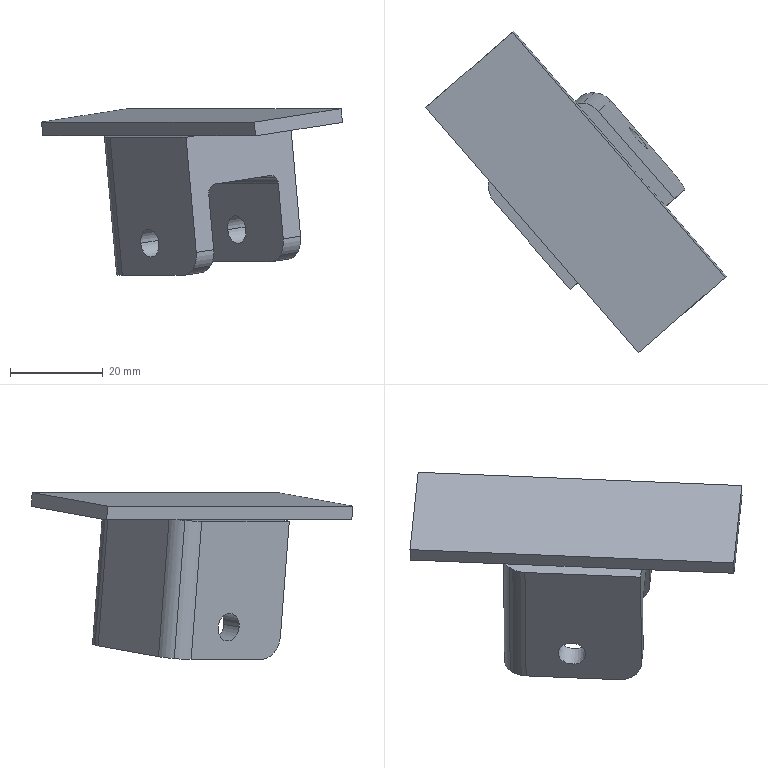Part | SolidWorks | features BaseBody 1 | 1 solid | 34 faces | box 64.897 x 69.371 x 35.986 mm | volume 22135 mm3 | plane 18 | cylinder 16 | commonest cylinder face diameters 10 x8 4 x4 6 x4
STEP:
#1=CARTESIAN_POINT('',(370.575,-213.244,-230.441));
#2=VERTEX_POINT('',#1);
#3=CARTESIAN_POINT('',(374.508,-217.775,-230.441));
#4=VERTEX_POINT('',#3);
#5=CARTESIAN_POINT('',(372.541,-215.51,-230.441));
#6=DIRECTION('',(-0.7501,-0.6509,-0.1168));
#7=DIRECTION('',(0.6554,-0.7553,0.));
#8=AXIS2_PLACEMENT_3D('',#5,#6,#7);
#9=CIRCLE('',#8,3.);
#10=EDGE_CURVE('',#2,#4,#9,.T.);
#11=ORIENTED_EDGE('',*,*,#10,.F.);
#12=CARTESIAN_POINT('',(366.824,-216.499,-231.025));
#13=VERTEX_POINT('',#12);
#14=CARTESIAN_POINT('',(389.327,-196.97,-227.522));
#15=DIRECTION('',(-0.7501,-0.6509,-0.1168));
#16=VECTOR('',#15,1000.);
#17=LINE('',#14,#16);
#18=EDGE_CURVE('',#2,#13,#17,.T.);
#19=ORIENTED_EDGE('',*,*,#18,.T.);
#20=CARTESIAN_POINT('',(370.757,-221.03,-231.025));
#21=VERTEX_POINT('',#20);
#22=CARTESIAN_POINT('',(368.791,-218.764,-231.025));
#23=DIRECTION('',(0.7501,0.6509,0.1168));
#24=DIRECTION('',(0.6554,-0.7553,0.));
#25=AXIS2_PLACEMENT_3D('',#22,#23,#24);
#26=CIRCLE('',#25,3.);
#27=EDGE_CURVE('',#21,#13,#26,.T.);
#28=ORIENTED_EDGE('',*,*,#27,.F.);
#29=CARTESIAN_POINT('',(393.26,-201.502,-227.522));
#30=DIRECTION('',(-0.7501,-0.6509,-0.1168));
#31=VECTOR('',#30,1000.);
#32=LINE('',#29,#31);
#33=EDGE_CURVE('',#4,#21,#32,.T.);
#34=ORIENTED_EDGE('',*,*,#33,.F.);
#35=EDGE_LOOP('',(#11,#19,#28,#34));
#36=FACE_OUTER_BOUND('',#35,.T.);
#37=CARTESIAN_POINT('',(391.293,-199.236,-227.522));
#38=DIRECTION('',(-0.7501,-0.6509,-0.1168));
#39=DIRECTION('',(0.6554,-0.7553,0.));
#40=AXIS2_PLACEMENT_3D('',#37,#38,#39);
#41=CYLINDRICAL_SURFACE('',#40,3.);
#42=ADVANCED_FACE('',(#36),#41,.F.);
#43=CARTESIAN_POINT('',(389.327,-196.97,-227.522));
#44=VERTEX_POINT('',#43);
#45=CARTESIAN_POINT('',(393.26,-201.502,-227.522));
#46=VERTEX_POINT('',#45);
#47=CARTESIAN_POINT('',(391.293,-199.236,-227.522));
#48=DIRECTION('',(-0.7501,-0.6509,-0.1168));
#49=DIRECTION('',(0.6554,-0.7553,0.));
#50=AXIS2_PLACEMENT_3D('',#47,#48,#49);
#51=CIRCLE('',#50,3.);
#52=EDGE_CURVE('',#44,#46,#51,.T.);
#53=ORIENTED_EDGE('',*,*,#52,.F.);
#54=CARTESIAN_POINT('',(385.577,-200.225,-228.106));
#55=VERTEX_POINT('',#54);
#56=CARTESIAN_POINT('',(389.327,-196.97,-227.522));
#57=DIRECTION('',(-0.7501,-0.6509,-0.1168));
#58=VECTOR('',#57,1000.);
#59=LINE('',#56,#58);
#60=EDGE_CURVE('',#44,#55,#59,.T.);
#61=ORIENTED_EDGE('',*,*,#60,.T.);
#62=CARTESIAN_POINT('',(389.509,-204.756,-228.106));
#63=VERTEX_POINT('',#62);
#64=CARTESIAN_POINT('',(387.543,-202.491,-228.106));
#65=DIRECTION('',(0.7501,0.6509,0.1168));
#66=DIRECTION('',(0.6554,-0.7553,0.));
#67=AXIS2_PLACEMENT_3D('',#64,#65,#66);
#68=CIRCLE('',#67,3.);
#69=EDGE_CURVE('',#63,#55,#68,.T.);
#70=ORIENTED_EDGE('',*,*,#69,.F.);
#71=CARTESIAN_POINT('',(393.26,-201.502,-227.522));
#72=DIRECTION('',(-0.7501,-0.6509,-0.1168));
#73=VECTOR('',#72,1000.);
#74=LINE('',#71,#73);
#75=EDGE_CURVE('',#46,#63,#74,.T.);
#76=ORIENTED_EDGE('',*,*,#75,.F.);
#77=EDGE_LOOP('',(#53,#61,#70,#76));
#78=FACE_OUTER_BOUND('',#77,.T.);
#79=CARTESIAN_POINT('',(391.293,-199.236,-227.522));
#80=DIRECTION('',(-0.7501,-0.6509,-0.1168));
#81=DIRECTION('',(0.6554,-0.7553,0.));
#82=AXIS2_PLACEMENT_3D('',#79,#80,#81);
#83=CYLINDRICAL_SURFACE('',#82,3.);
#84=ADVANCED_FACE('',(#78),#83,.F.);
#85=CARTESIAN_POINT('',(396.492,-214.585,-218.174));
#86=VERTEX_POINT('',#85);
#87=CARTESIAN_POINT('',(395.928,-215.074,-216.838));
#88=VERTEX_POINT('',#87);
#89=CARTESIAN_POINT('',(394.992,-215.887,-218.408));
#90=DIRECTION('',(0.6554,-0.7553,0.));
#91=DIRECTION('',(0.468,0.4062,0.7848));
#92=AXIS2_PLACEMENT_3D('',#89,#90,#91);
#93=CIRCLE('',#92,2.);
#94=EDGE_CURVE('',#86,#88,#93,.T.);
#95=ORIENTED_EDGE('',*,*,#94,.T.);
#96=CARTESIAN_POINT('',(379.543,-196.193,-216.838));
#97=VERTEX_POINT('',#96);
#98=CARTESIAN_POINT('',(395.928,-215.074,-216.838));
#99=DIRECTION('',(-0.6554,0.7553,0.));
#100=VECTOR('',#99,1000.);
#101=LINE('',#98,#100);
#102=EDGE_CURVE('',#88,#97,#101,.T.);
#103=ORIENTED_EDGE('',*,*,#102,.T.);
#104=CARTESIAN_POINT('',(380.107,-195.703,-218.174));
#105=VERTEX_POINT('',#104);
#106=CARTESIAN_POINT('',(378.607,-197.005,-218.408));
#107=DIRECTION('',(0.6554,-0.7553,0.));
#108=DIRECTION('',(0.468,0.4062,0.7848));
#109=AXIS2_PLACEMENT_3D('',#106,#107,#108);
#110=CIRCLE('',#109,2.);
#111=EDGE_CURVE('',#105,#97,#110,.T.);
#112=ORIENTED_EDGE('',*,*,#111,.F.);
#113=CARTESIAN_POINT('',(396.492,-214.585,-218.174));
#114=DIRECTION('',(0.6554,-0.7553,0.));
#115=VECTOR('',#114,1000.);
#116=LINE('',#113,#115);
#117=EDGE_CURVE('',#105,#86,#116,.T.);
#118=ORIENTED_EDGE('',*,*,#117,.T.);
#119=EDGE_LOOP('',(#95,#103,#112,#118));
#120=FACE_OUTER_BOUND('',#119,.T.);
#121=CARTESIAN_POINT('',(394.992,-215.887,-218.408));
#122=DIRECTION('',(-0.6554,0.7553,0.));
#123=DIRECTION('',(0.468,0.4062,0.7848));
#124=AXIS2_PLACEMENT_3D('',#121,#122,#123);
#125=CYLINDRICAL_SURFACE('',#124,2.);
#126=ADVANCED_FACE('',(#120),#125,.F.);
#127=CARTESIAN_POINT('',(382.814,-226.455,-218.29));
#128=VERTEX_POINT('',#127);
#129=CARTESIAN_POINT('',(381.805,-227.331,-219.037));
#130=VERTEX_POINT('',#129);
#131=CARTESIAN_POINT('',(382.991,-226.302,-220.276));
#132=DIRECTION('',(0.6554,-0.7553,0.));
#133=DIRECTION('',(-0.5928,-0.5144,0.6197));
#134=AXIS2_PLACEMENT_3D('',#131,#132,#133);
#135=CIRCLE('',#134,2.);
#136=EDGE_CURVE('',#128,#130,#135,.T.);
#137=ORIENTED_EDGE('',*,*,#136,.T.);
#138=CARTESIAN_POINT('',(365.42,-208.449,-219.037));
#139=VERTEX_POINT('',#138);
#140=CARTESIAN_POINT('',(381.805,-227.331,-219.037));
#141=DIRECTION('',(-0.6554,0.7553,0.));
#142=VECTOR('',#141,1000.);
#143=LINE('',#140,#142);
#144=EDGE_CURVE('',#130,#139,#143,.T.);
#145=ORIENTED_EDGE('',*,*,#144,.T.);
#146=CARTESIAN_POINT('',(366.429,-207.574,-218.29));
#147=VERTEX_POINT('',#146);
#148=CARTESIAN_POINT('',(366.605,-207.421,-220.276));
#149=DIRECTION('',(0.6554,-0.7553,0.));
#150=DIRECTION('',(-0.5928,-0.5144,0.6197));
#151=AXIS2_PLACEMENT_3D('',#148,#149,#150);
#152=CIRCLE('',#151,2.);
#153=EDGE_CURVE('',#147,#139,#152,.T.);
#154=ORIENTED_EDGE('',*,*,#153,.F.);
#155=CARTESIAN_POINT('',(382.814,-226.455,-218.29));
#156=DIRECTION('',(0.6554,-0.7553,0.));
#157=VECTOR('',#156,1000.);
#158=LINE('',#155,#157);
#159=EDGE_CURVE('',#147,#128,#158,.T.);
#160=ORIENTED_EDGE('',*,*,#159,.T.);
#161=EDGE_LOOP('',(#137,#145,#154,#160));
#162=FACE_OUTER_BOUND('',#161,.T.);
#163=CARTESIAN_POINT('',(382.991,-226.302,-220.276));
#164=DIRECTION('',(-0.6554,0.7553,0.));
#165=DIRECTION('',(-0.5928,-0.5144,0.6197));
#166=AXIS2_PLACEMENT_3D('',#163,#164,#165);
#167=CYLINDRICAL_SURFACE('',#166,2.);
#168=ADVANCED_FACE('',(#162),#167,.F.);
#169=CARTESIAN_POINT('',(378.799,-229.94,-233.011));
#170=VERTEX_POINT('',#169);
#171=CARTESIAN_POINT('',(378.151,-228.563,-236.523));
#172=VERTEX_POINT('',#171);
#173=CARTESIAN_POINT('',(375.521,-226.164,-233.011));
#174=DIRECTION('',(0.7501,0.6509,0.1168));
#175=DIRECTION('',(0.5258,-0.4799,-0.7023));
#176=AXIS2_PLACEMENT_3D('',#173,#174,#175);
#177=CIRCLE('',#176,5.);
#178=EDGE_CURVE('',#170,#172,#177,.T.);
#179=ORIENTED_EDGE('',*,*,#178,.T.);
#180=CARTESIAN_POINT('',(381.901,-225.309,-235.939));
#181=VERTEX_POINT('',#180);
#182=CARTESIAN_POINT('',(378.151,-228.563,-236.523));
#183=DIRECTION('',(0.7501,0.6509,0.1168));
#184=VECTOR('',#183,1000.);
#185=LINE('',#182,#184);
#186=EDGE_CURVE('',#172,#181,#185,.T.);
#187=ORIENTED_EDGE('',*,*,#186,.T.);
#188=CARTESIAN_POINT('',(382.549,-226.685,-232.428));
#189=VERTEX_POINT('',#188);
#190=CARTESIAN_POINT('',(379.272,-222.909,-232.428));
#191=DIRECTION('',(-0.7501,-0.6509,-0.1168));
#192=DIRECTION('',(0.5258,-0.4799,-0.7023));
#193=AXIS2_PLACEMENT_3D('',#190,#191,#192);
#194=CIRCLE('',#193,5.);
#195=EDGE_CURVE('',#181,#189,#194,.T.);
#196=ORIENTED_EDGE('',*,*,#195,.T.);
#197=CARTESIAN_POINT('',(378.799,-229.94,-233.011));
#198=DIRECTION('',(-0.7501,-0.6509,-0.1168));
#199=VECTOR('',#198,1000.);
#200=LINE('',#197,#199);
#201=EDGE_CURVE('',#189,#170,#200,.T.);
#202=ORIENTED_EDGE('',*,*,#201,.T.);
#203=EDGE_LOOP('',(#179,#187,#196,#202));
#204=FACE_OUTER_BOUND('',#203,.T.);
#205=CARTESIAN_POINT('',(375.521,-226.164,-233.011));
#206=DIRECTION('',(0.7501,0.6509,0.1168));
#207=DIRECTION('',(0.5258,-0.4799,-0.7023));
#208=AXIS2_PLACEMENT_3D('',#205,#206,#207);
#209=CYLINDRICAL_SURFACE('',#208,5.);
#210=ADVANCED_FACE('',(#204),#209,.T.);
#211=CARTESIAN_POINT('',(397.551,-213.666,-230.092));
#212=VERTEX_POINT('',#211);
#213=CARTESIAN_POINT('',(396.903,-212.29,-233.603));
#214=VERTEX_POINT('',#213);
#215=CARTESIAN_POINT('',(394.274,-209.89,-230.092));
#216=DIRECTION('',(0.7501,0.6509,0.1168));
#217=DIRECTION('',(0.5258,-0.4799,-0.7023));
#218=AXIS2_PLACEMENT_3D('',#215,#216,#217);
#219=CIRCLE('',#218,5.);
#220=EDGE_CURVE('',#212,#214,#219,.T.);
#221=ORIENTED_EDGE('',*,*,#220,.T.);
#222=CARTESIAN_POINT('',(400.653,-209.035,-233.02));
#223=VERTEX_POINT('',#222);
#224=CARTESIAN_POINT('',(378.151,-228.563,-236.523));
#225=DIRECTION('',(0.7501,0.6509,0.1168));
#226=VECTOR('',#225,1000.);
#227=LINE('',#224,#226);
#228=EDGE_CURVE('',#214,#223,#227,.T.);
#229=ORIENTED_EDGE('',*,*,#228,.T.);
#230=CARTESIAN_POINT('',(401.301,-210.412,-229.508));
#231=VERTEX_POINT('',#230);
#232=CARTESIAN_POINT('',(398.024,-206.635,-229.508));
#233=DIRECTION('',(-0.7501,-0.6509,-0.1168));
#234=DIRECTION('',(0.5258,-0.4799,-0.7023));
#235=AXIS2_PLACEMENT_3D('',#232,#233,#234);
#236=CIRCLE('',#235,5.);
#237=EDGE_CURVE('',#223,#231,#236,.T.);
#238=ORIENTED_EDGE('',*,*,#237,.T.);
#239=CARTESIAN_POINT('',(378.799,-229.94,-233.011));
#240=DIRECTION('',(-0.7501,-0.6509,-0.1168));
#241=VECTOR('',#240,1000.);
#242=LINE('',#239,#241);
#243=EDGE_CURVE('',#231,#212,#242,.T.);
#244=ORIENTED_EDGE('',*,*,#243,.T.);
#245=EDGE_LOOP('',(#221,#229,#238,#244));
#246=FACE_OUTER_BOUND('',#245,.T.);
#247=CARTESIAN_POINT('',(375.521,-226.164,-233.011));
#248=DIRECTION('',(0.7501,0.6509,0.1168));
#249=DIRECTION('',(0.5258,-0.4799,-0.7023));
#250=AXIS2_PLACEMENT_3D('',#247,#248,#249);
#251=CYLINDRICAL_SURFACE('',#250,5.);
#252=ADVANCED_FACE('',(#246),#251,.T.);
#253=CARTESIAN_POINT('',(363.327,-203.645,-237.393));
#254=VERTEX_POINT('',#253);
#255=CARTESIAN_POINT('',(361.635,-207.052,-237.806));
#256=VERTEX_POINT('',#255);
#257=CARTESIAN_POINT('',(366.604,-207.421,-237.393));
#258=DIRECTION('',(-0.0882,-0.07654,0.9932));
#259=DIRECTION('',(-0.9939,0.07376,-0.08257));
#260=AXIS2_PLACEMENT_3D('',#257,#258,#259);
#261=CIRCLE('',#260,5.);
#262=EDGE_CURVE('',#254,#256,#261,.T.);
#263=ORIENTED_EDGE('',*,*,#262,.T.);
#264=CARTESIAN_POINT('',(358.989,-209.349,-208.012));
#265=VERTEX_POINT('',#264);
#266=CARTESIAN_POINT('',(360.974,-207.626,-230.358));
#267=DIRECTION('',(-0.0882,-0.07654,0.9932));
#268=VECTOR('',#267,1000.);
#269=LINE('',#266,#268);
#270=EDGE_CURVE('',#256,#265,#269,.T.);
#271=ORIENTED_EDGE('',*,*,#270,.T.);
#272=CARTESIAN_POINT('',(359.245,-208.074,-207.891));
#273=VERTEX_POINT('',#272);
#274=CARTESIAN_POINT('',(363.958,-209.717,-207.599));
#275=DIRECTION('',(0.0882,0.07654,-0.9932));
#276=DIRECTION('',(-0.9939,0.07376,-0.08257));
#277=AXIS2_PLACEMENT_3D('',#274,#275,#276);
#278=CIRCLE('',#277,5.);
#279=EDGE_CURVE('',#265,#273,#278,.T.);
#280=ORIENTED_EDGE('',*,*,#279,.T.);
#281=CARTESIAN_POINT('',(360.681,-205.941,-207.599));
#282=VERTEX_POINT('',#281);
#283=CARTESIAN_POINT('',(363.958,-209.717,-207.599));
#284=DIRECTION('',(0.0882,0.07654,-0.9932));
#285=DIRECTION('',(-0.9939,0.07376,-0.08257));
#286=AXIS2_PLACEMENT_3D('',#283,#284,#285);
#287=CIRCLE('',#286,5.);
#288=EDGE_CURVE('',#273,#282,#287,.T.);
#289=ORIENTED_EDGE('',*,*,#288,.T.);
#290=CARTESIAN_POINT('',(362.666,-204.219,-229.945));
#291=DIRECTION('',(0.0882,0.07654,-0.9932));
#292=VECTOR('',#291,1000.);
#293=LINE('',#290,#292);
#294=EDGE_CURVE('',#282,#254,#293,.T.);
#295=ORIENTED_EDGE('',*,*,#294,.T.);
#296=EDGE_LOOP('',(#263,#271,#280,#289,#295));
#297=FACE_OUTER_BOUND('',#296,.T.);
#298=CARTESIAN_POINT('',(365.943,-207.995,-229.945));
#299=DIRECTION('',(-0.0882,-0.07654,0.9932));
#300=DIRECTION('',(-0.9939,0.07376,-0.08257));
#301=AXIS2_PLACEMENT_3D('',#298,#299,#300);
#302=CYLINDRICAL_SURFACE('',#301,5.);
#303=ADVANCED_FACE('',(#297),#302,.T.);
#304=CARTESIAN_POINT('',(385.357,-191.148,-234.474));
#305=VERTEX_POINT('',#304);
#306=CARTESIAN_POINT('',(381.941,-189.431,-234.645));
#307=VERTEX_POINT('',#306);
#308=CARTESIAN_POINT('',(381.606,-194.402,-235.058));
#309=DIRECTION('',(-0.0882,-0.07654,0.9932));
#310=DIRECTION('',(0.06694,0.9943,0.08257));
#311=AXIS2_PLACEMENT_3D('',#308,#309,#310);
#312=CIRCLE('',#311,5.);
#313=EDGE_CURVE('',#305,#307,#312,.T.);
#314=ORIENTED_EDGE('',*,*,#313,.T.);
#315=CARTESIAN_POINT('',(379.295,-191.727,-204.85));
#316=VERTEX_POINT('',#315);
#317=CARTESIAN_POINT('',(381.279,-190.005,-227.196));
#318=DIRECTION('',(-0.0882,-0.07654,0.9932));
#319=VECTOR('',#318,1000.);
#320=LINE('',#317,#319);
#321=EDGE_CURVE('',#307,#316,#320,.T.);
#322=ORIENTED_EDGE('',*,*,#321,.T.);
#323=CARTESIAN_POINT('',(382.711,-193.444,-204.679));
#324=VERTEX_POINT('',#323);
#325=CARTESIAN_POINT('',(378.96,-196.698,-205.263));
#326=DIRECTION('',(0.0882,0.07654,-0.9932));
#327=DIRECTION('',(0.06694,0.9943,0.08257));
#328=AXIS2_PLACEMENT_3D('',#325,#326,#327);
#329=CIRCLE('',#328,5.);
#330=EDGE_CURVE('',#316,#324,#329,.T.);
#331=ORIENTED_EDGE('',*,*,#330,.T.);
#332=CARTESIAN_POINT('',(384.695,-191.722,-227.025));
#333=DIRECTION('',(0.0882,0.07654,-0.9932));
#334=VECTOR('',#333,1000.);
#335=LINE('',#332,#334);
#336=EDGE_CURVE('',#324,#305,#335,.T.);
#337=ORIENTED_EDGE('',*,*,#336,.T.);
#338=EDGE_LOOP('',(#314,#322,#331,#337));
#339=FACE_OUTER_BOUND('',#338,.T.);
#340=CARTESIAN_POINT('',(380.945,-194.976,-227.609));
#341=DIRECTION('',(-0.0882,-0.07654,0.9932));
#342=DIRECTION('',(0.06694,0.9943,0.08257));
#343=AXIS2_PLACEMENT_3D('',#340,#341,#342);
#344=CYLINDRICAL_SURFACE('',#343,5.);
#345=ADVANCED_FACE('',(#339),#344,.T.);
#346=ORIENTED_EDGE('',*,*,#27,.T.);
#347=CARTESIAN_POINT('',(368.791,-218.764,-231.025));
#348=DIRECTION('',(0.7501,0.6509,0.1168));
#349=DIRECTION('',(0.6554,-0.7553,0.));
#350=AXIS2_PLACEMENT_3D('',#347,#348,#349);
#351=CIRCLE('',#350,3.);
#352=EDGE_CURVE('',#13,#21,#351,.T.);
#353=ORIENTED_EDGE('',*,*,#352,.T.);
#354=EDGE_LOOP('',(#346,#353));
#355=FACE_BOUND('',#354,.T.);
#356=ORIENTED_EDGE('',*,*,#178,.F.);
#357=CARTESIAN_POINT('',(376.594,-231.854,-208.183));
#358=VERTEX_POINT('',#357);
#359=CARTESIAN_POINT('',(376.594,-231.854,-208.183));
#360=DIRECTION('',(0.0882,0.07654,-0.9932));
#361=VECTOR('',#360,1000.);
#362=LINE('',#359,#361);
#363=EDGE_CURVE('',#358,#170,#362,.T.);
#364=ORIENTED_EDGE('',*,*,#363,.F.);
#365=CARTESIAN_POINT('',(360.208,-212.972,-208.183));
#366=VERTEX_POINT('',#365);
#367=CARTESIAN_POINT('',(356.931,-209.196,-208.183));
#368=DIRECTION('',(0.6554,-0.7553,0.));
#369=VECTOR('',#368,1000.);
#370=LINE('',#367,#369);
#371=EDGE_CURVE('',#366,#358,#370,.T.);
#372=ORIENTED_EDGE('',*,*,#371,.F.);
#373=CARTESIAN_POINT('',(362.854,-210.676,-237.977));
#374=VERTEX_POINT('',#373);
#375=CARTESIAN_POINT('',(362.192,-211.25,-230.529));
#376=DIRECTION('',(-0.0882,-0.07654,0.9932));
#377=VECTOR('',#376,1000.);
#378=LINE('',#375,#377);
#379=EDGE_CURVE('',#374,#366,#378,.T.);
#380=ORIENTED_EDGE('',*,*,#379,.F.);
#381=CARTESIAN_POINT('',(375.962,-225.781,-237.977));
#382=VERTEX_POINT('',#381);
#383=CARTESIAN_POINT('',(379.24,-229.557,-237.977));
#384=DIRECTION('',(-0.6554,0.7553,0.));
#385=VECTOR('',#384,1000.);
#386=LINE('',#383,#385);
#387=EDGE_CURVE('',#382,#374,#386,.T.);
#388=ORIENTED_EDGE('',*,*,#387,.F.);
#389=CARTESIAN_POINT('',(375.521,-226.164,-233.011));
#390=DIRECTION('',(0.7501,0.6509,0.1168));
#391=DIRECTION('',(0.5258,-0.4799,-0.7023));
#392=AXIS2_PLACEMENT_3D('',#389,#390,#391);
#393=CIRCLE('',#392,5.);
#394=EDGE_CURVE('',#172,#382,#393,.T.);
#395=ORIENTED_EDGE('',*,*,#394,.F.);
#396=EDGE_LOOP('',(#356,#364,#372,#380,#388,#395));
#397=FACE_OUTER_BOUND('',#396,.T.);
#398=CARTESIAN_POINT('',(368.085,-219.377,-223.08));
#399=DIRECTION('',(0.7501,0.6509,0.1168));
#400=DIRECTION('',(-0.6554,0.7553,0.));
#401=AXIS2_PLACEMENT_3D('',#398,#399,#400);
#402=PLANE('',#401);
#403=ADVANCED_FACE('',(#355,#397),#402,.F.);
#404=CARTESIAN_POINT('',(391.293,-199.236,-227.522));
#405=DIRECTION('',(-0.7501,-0.6509,-0.1168));
#406=DIRECTION('',(0.6554,-0.7553,0.));
#407=AXIS2_PLACEMENT_3D('',#404,#405,#406);
#408=CIRCLE('',#407,3.);
#409=EDGE_CURVE('',#46,#44,#408,.T.);
#410=ORIENTED_EDGE('',*,*,#409,.T.);
#411=ORIENTED_EDGE('',*,*,#52,.T.);
#412=EDGE_LOOP('',(#410,#411));
#413=FACE_BOUND('',#412,.T.);
#414=CARTESIAN_POINT('',(398.465,-206.253,-234.474));
#415=VERTEX_POINT('',#414);
#416=CARTESIAN_POINT('',(398.024,-206.635,-229.508));
#417=DIRECTION('',(-0.7501,-0.6509,-0.1168));
#418=DIRECTION('',(0.5258,-0.4799,-0.7023));
#419=AXIS2_PLACEMENT_3D('',#416,#417,#418);
#420=CIRCLE('',#419,5.);
#421=EDGE_CURVE('',#415,#223,#420,.T.);
#422=ORIENTED_EDGE('',*,*,#421,.F.);
#423=CARTESIAN_POINT('',(401.742,-210.029,-234.474));
#424=DIRECTION('',(-0.6554,0.7553,0.));
#425=VECTOR('',#424,1000.);
#426=LINE('',#423,#425);
#427=EDGE_CURVE('',#415,#305,#426,.T.);
#428=ORIENTED_EDGE('',*,*,#427,.T.);
#429=ORIENTED_EDGE('',*,*,#336,.F.);
#430=CARTESIAN_POINT('',(399.096,-212.325,-204.679));
#431=VERTEX_POINT('',#430);
#432=CARTESIAN_POINT('',(379.434,-189.667,-204.679));
#433=DIRECTION('',(0.6554,-0.7553,0.));
#434=VECTOR('',#433,1000.);
#435=LINE('',#432,#434);
#436=EDGE_CURVE('',#324,#431,#435,.T.);
#437=ORIENTED_EDGE('',*,*,#436,.T.);
#438=CARTESIAN_POINT('',(399.096,-212.325,-204.679));
#439=DIRECTION('',(0.0882,0.07654,-0.9932));
#440=VECTOR('',#439,1000.);
#441=LINE('',#438,#440);
#442=EDGE_CURVE('',#431,#231,#441,.T.);
#443=ORIENTED_EDGE('',*,*,#442,.T.);
#444=ORIENTED_EDGE('',*,*,#237,.F.);
#445=EDGE_LOOP('',(#422,#428,#429,#437,#443,#444));
#446=FACE_OUTER_BOUND('',#445,.T.);
#447=CARTESIAN_POINT('',(390.588,-199.848,-219.577));
#448=DIRECTION('',(0.7501,0.6509,0.1168));
#449=DIRECTION('',(-0.6554,0.7553,0.));
#450=AXIS2_PLACEMENT_3D('',#447,#448,#449);
#451=PLANE('',#450);
#452=ADVANCED_FACE('',(#413,#446),#451,.T.);
#453=ORIENTED_EDGE('',*,*,#321,.F.);
#454=CARTESIAN_POINT('',(378.329,-190.626,-235.058));
#455=VERTEX_POINT('',#454);
#456=CARTESIAN_POINT('',(381.606,-194.402,-235.058));
#457=DIRECTION('',(-0.0882,-0.07654,0.9932));
#458=DIRECTION('',(0.06694,0.9943,0.08257));
#459=AXIS2_PLACEMENT_3D('',#456,#457,#458);
#460=CIRCLE('',#459,5.);
#461=EDGE_CURVE('',#307,#455,#460,.T.);
#462=ORIENTED_EDGE('',*,*,#461,.T.);
#463=CARTESIAN_POINT('',(375.683,-192.922,-205.263));
#464=VERTEX_POINT('',#463);
#465=CARTESIAN_POINT('',(377.667,-191.2,-227.609));
#466=DIRECTION('',(-0.0882,-0.07654,0.9932));
#467=VECTOR('',#466,1000.);
#468=LINE('',#465,#467);
#469=EDGE_CURVE('',#455,#464,#468,.T.);
#470=ORIENTED_EDGE('',*,*,#469,.T.);
#471=CARTESIAN_POINT('',(377.997,-191.801,-204.971));
#472=VERTEX_POINT('',#471);
#473=CARTESIAN_POINT('',(378.96,-196.698,-205.263));
#474=DIRECTION('',(0.0882,0.07654,-0.9932));
#475=DIRECTION('',(0.06694,0.9943,0.08257));
#476=AXIS2_PLACEMENT_3D('',#473,#474,#475);
#477=CIRCLE('',#476,5.);
#478=EDGE_CURVE('',#464,#472,#477,.T.);
#479=ORIENTED_EDGE('',*,*,#478,.T.);
#480=CARTESIAN_POINT('',(378.96,-196.698,-205.263));
#481=DIRECTION('',(0.0882,0.07654,-0.9932));
#482=DIRECTION('',(0.06694,0.9943,0.08257));
#483=AXIS2_PLACEMENT_3D('',#480,#481,#482);
#484=CIRCLE('',#483,5.);
#485=EDGE_CURVE('',#472,#316,#484,.T.);
#486=ORIENTED_EDGE('',*,*,#485,.T.);
#487=EDGE_LOOP('',(#453,#462,#470,#479,#486));
#488=FACE_OUTER_BOUND('',#487,.T.);
#489=CARTESIAN_POINT('',(380.945,-194.976,-227.609));
#490=DIRECTION('',(-0.0882,-0.07654,0.9932));
#491=DIRECTION('',(0.06694,0.9943,0.08257));
#492=AXIS2_PLACEMENT_3D('',#489,#490,#491);
#493=CYLINDRICAL_SURFACE('',#492,5.);
#494=ADVANCED_FACE('',(#488),#493,.T.);
#495=ORIENTED_EDGE('',*,*,#294,.F.);
#496=CARTESIAN_POINT('',(356.931,-209.196,-208.183));
#497=DIRECTION('',(0.7501,0.6509,0.1168));
#498=VECTOR('',#497,1000.);
#499=LINE('',#496,#498);
#500=EDGE_CURVE('',#282,#464,#499,.T.);
#501=ORIENTED_EDGE('',*,*,#500,.T.);
#502=ORIENTED_EDGE('',*,*,#469,.F.);
#503=CARTESIAN_POINT('',(359.577,-206.9,-237.977));
#504=DIRECTION('',(0.7501,0.6509,0.1168));
#505=VECTOR('',#504,1000.);
#506=LINE('',#503,#505);
#507=EDGE_CURVE('',#254,#455,#506,.T.);
#508=ORIENTED_EDGE('',*,*,#507,.F.);
#509=EDGE_LOOP('',(#495,#501,#502,#508));
#510=FACE_OUTER_BOUND('',#509,.T.);
#511=CARTESIAN_POINT('',(359.577,-206.9,-237.977));
#512=DIRECTION('',(-0.6554,0.7553,0.));
#513=DIRECTION('',(-0.0882,-0.07654,0.9932));
#514=AXIS2_PLACEMENT_3D('',#511,#512,#513);
#515=PLANE('',#514);
#516=ADVANCED_FACE('',(#510),#515,.T.);
#517=ORIENTED_EDGE('',*,*,#270,.F.);
#518=CARTESIAN_POINT('',(366.604,-207.421,-237.393));
#519=DIRECTION('',(-0.0882,-0.07654,0.9932));
#520=DIRECTION('',(-0.9939,0.07376,-0.08257));
#521=AXIS2_PLACEMENT_3D('',#518,#519,#520);
#522=CIRCLE('',#521,5.);
#523=EDGE_CURVE('',#256,#374,#522,.T.);
#524=ORIENTED_EDGE('',*,*,#523,.T.);
#525=ORIENTED_EDGE('',*,*,#379,.T.);
#526=CARTESIAN_POINT('',(363.958,-209.717,-207.599));
#527=DIRECTION('',(0.0882,0.07654,-0.9932));
#528=DIRECTION('',(-0.9939,0.07376,-0.08257));
#529=AXIS2_PLACEMENT_3D('',#526,#527,#528);
#530=CIRCLE('',#529,5.);
#531=EDGE_CURVE('',#366,#265,#530,.T.);
#532=ORIENTED_EDGE('',*,*,#531,.T.);
#533=EDGE_LOOP('',(#517,#524,#525,#532));
#534=FACE_OUTER_BOUND('',#533,.T.);
#535=CARTESIAN_POINT('',(365.943,-207.995,-229.945));
#536=DIRECTION('',(-0.0882,-0.07654,0.9932));
#537=DIRECTION('',(-0.9939,0.07376,-0.08257));
#538=AXIS2_PLACEMENT_3D('',#535,#536,#537);
#539=CYLINDRICAL_SURFACE('',#538,5.);
#540=ADVANCED_FACE('',(#534),#539,.T.);
#541=ORIENTED_EDGE('',*,*,#201,.F.);
#542=CARTESIAN_POINT('',(381.491,-227.604,-220.51));
#543=VERTEX_POINT('',#542);
#544=CARTESIAN_POINT('',(381.82,-227.318,-224.213));
#545=DIRECTION('',(-0.0882,-0.07654,0.9932));
#546=VECTOR('',#545,1000.);
#547=LINE('',#544,#546);
#548=EDGE_CURVE('',#189,#543,#547,.T.);
#549=ORIENTED_EDGE('',*,*,#548,.T.);
#550=CARTESIAN_POINT('',(382.991,-226.302,-220.276));
#551=DIRECTION('',(0.6554,-0.7553,0.));
#552=DIRECTION('',(-0.5928,-0.5144,0.6197));
#553=AXIS2_PLACEMENT_3D('',#550,#551,#552);
#554=CIRCLE('',#553,2.);
#555=EDGE_CURVE('',#130,#543,#554,.T.);
#556=ORIENTED_EDGE('',*,*,#555,.F.);
#557=ORIENTED_EDGE('',*,*,#136,.F.);
#558=CARTESIAN_POINT('',(394.816,-216.04,-216.421));
#559=VERTEX_POINT('',#558);
#560=CARTESIAN_POINT('',(379.439,-229.384,-218.815));
#561=DIRECTION('',(0.7501,0.6509,0.1168));
#562=VECTOR('',#561,1000.);
#563=LINE('',#560,#562);
#564=EDGE_CURVE('',#128,#559,#563,.T.);
#565=ORIENTED_EDGE('',*,*,#564,.T.);
#566=CARTESIAN_POINT('',(394.992,-215.887,-218.408));
#567=DIRECTION('',(0.6554,-0.7553,0.));
#568=DIRECTION('',(0.468,0.4062,0.7848));
#569=AXIS2_PLACEMENT_3D('',#566,#567,#568);
#570=CIRCLE('',#569,2.);
#571=EDGE_CURVE('',#88,#559,#570,.T.);
#572=ORIENTED_EDGE('',*,*,#571,.F.);
#573=ORIENTED_EDGE('',*,*,#94,.F.);
#574=CARTESIAN_POINT('',(395.831,-215.159,-210.725));
#575=DIRECTION('',(0.0882,0.07654,-0.9932));
#576=VECTOR('',#575,1000.);
#577=LINE('',#574,#576);
#578=EDGE_CURVE('',#86,#212,#577,.T.);
#579=ORIENTED_EDGE('',*,*,#578,.T.);
#580=ORIENTED_EDGE('',*,*,#243,.F.);
#581=ORIENTED_EDGE('',*,*,#442,.F.);
#582=CARTESIAN_POINT('',(397.221,-213.953,-204.971));
#583=VERTEX_POINT('',#582);
#584=CARTESIAN_POINT('',(376.594,-231.854,-208.183));
#585=DIRECTION('',(0.7501,0.6509,0.1168));
#586=VECTOR('',#585,1000.);
#587=LINE('',#584,#586);
#588=EDGE_CURVE('',#583,#431,#587,.T.);
#589=ORIENTED_EDGE('',*,*,#588,.F.);
#590=CARTESIAN_POINT('',(378.469,-230.226,-207.891));
#591=VERTEX_POINT('',#590);
#592=CARTESIAN_POINT('',(376.594,-231.854,-208.183));
#593=DIRECTION('',(0.7501,0.6509,0.1168));
#594=VECTOR('',#593,1000.);
#595=LINE('',#592,#594);
#596=EDGE_CURVE('',#591,#583,#595,.T.);
#597=ORIENTED_EDGE('',*,*,#596,.F.);
#598=CARTESIAN_POINT('',(376.594,-231.854,-208.183));
#599=DIRECTION('',(0.7501,0.6509,0.1168));
#600=VECTOR('',#599,1000.);
#601=LINE('',#598,#600);
#602=EDGE_CURVE('',#358,#591,#601,.T.);
#603=ORIENTED_EDGE('',*,*,#602,.F.);
#604=ORIENTED_EDGE('',*,*,#363,.T.);
#605=EDGE_LOOP('',(#541,#549,#556,#557,#565,#572,#573,#579,#580,#581,#589,#597,#603,#604));
#606=FACE_OUTER_BOUND('',#605,.T.);
#607=CARTESIAN_POINT('',(376.594,-231.854,-208.183));
#608=DIRECTION('',(0.6554,-0.7553,0.));
#609=DIRECTION('',(-0.0882,-0.07654,0.9932));
#610=AXIS2_PLACEMENT_3D('',#607,#608,#609);
#611=PLANE('',#610);
#612=ADVANCED_FACE('',(#606),#611,.T.);
#613=CARTESIAN_POINT('',(378.43,-197.158,-216.421));
#614=VERTEX_POINT('',#613);
#615=CARTESIAN_POINT('',(394.816,-216.04,-216.421));
#616=DIRECTION('',(-0.6554,0.7553,0.));
#617=VECTOR('',#616,1000.);
#618=LINE('',#615,#617);
#619=EDGE_CURVE('',#559,#614,#618,.T.);
#620=ORIENTED_EDGE('',*,*,#619,.F.);
#621=ORIENTED_EDGE('',*,*,#564,.F.);
#622=ORIENTED_EDGE('',*,*,#159,.F.);
#623=CARTESIAN_POINT('',(364.929,-208.875,-218.523));
#624=DIRECTION('',(0.7501,0.6509,0.1168));
#625=VECTOR('',#624,1000.);
#626=LINE('',#623,#625);
#627=EDGE_CURVE('',#147,#614,#626,.T.);
#628=ORIENTED_EDGE('',*,*,#627,.T.);
#629=EDGE_LOOP('',(#620,#621,#622,#628));
#630=FACE_OUTER_BOUND('',#629,.T.);
#631=CARTESIAN_POINT('',(381.314,-227.757,-218.523));
#632=DIRECTION('',(-0.0882,-0.07654,0.9932));
#633=DIRECTION('',(-0.6554,0.7553,0.));
#634=AXIS2_PLACEMENT_3D('',#631,#632,#633);
#635=PLANE('',#634);
#636=ADVANCED_FACE('',(#630),#635,.F.);
#637=ORIENTED_EDGE('',*,*,#228,.F.);
#638=CARTESIAN_POINT('',(394.715,-209.507,-235.058));
#639=VERTEX_POINT('',#638);
#640=CARTESIAN_POINT('',(394.274,-209.89,-230.092));
#641=DIRECTION('',(0.7501,0.6509,0.1168));
#642=DIRECTION('',(0.5258,-0.4799,-0.7023));
#643=AXIS2_PLACEMENT_3D('',#640,#641,#642);
#644=CIRCLE('',#643,5.);
#645=EDGE_CURVE('',#214,#639,#644,.T.);
#646=ORIENTED_EDGE('',*,*,#645,.T.);
#647=CARTESIAN_POINT('',(375.962,-225.781,-237.977));
#648=DIRECTION('',(0.7501,0.6509,0.1168));
#649=VECTOR('',#648,1000.);
#650=LINE('',#647,#649);
#651=EDGE_CURVE('',#639,#415,#650,.T.);
#652=ORIENTED_EDGE('',*,*,#651,.T.);
#653=ORIENTED_EDGE('',*,*,#421,.T.);
#654=EDGE_LOOP('',(#637,#646,#652,#653));
#655=FACE_OUTER_BOUND('',#654,.T.);
#656=CARTESIAN_POINT('',(375.521,-226.164,-233.011));
#657=DIRECTION('',(0.7501,0.6509,0.1168));
#658=DIRECTION('',(0.5258,-0.4799,-0.7023));
#659=AXIS2_PLACEMENT_3D('',#656,#657,#658);
#660=CYLINDRICAL_SURFACE('',#659,5.);
#661=ADVANCED_FACE('',(#655),#660,.T.);
#662=CARTESIAN_POINT('',(379.713,-222.526,-237.393));
#663=VERTEX_POINT('',#662);
#664=CARTESIAN_POINT('',(375.962,-225.781,-237.977));
#665=DIRECTION('',(0.7501,0.6509,0.1168));
#666=VECTOR('',#665,1000.);
#667=LINE('',#664,#666);
#668=EDGE_CURVE('',#382,#663,#667,.T.);
#669=ORIENTED_EDGE('',*,*,#668,.F.);
#670=ORIENTED_EDGE('',*,*,#387,.T.);
#671=ORIENTED_EDGE('',*,*,#523,.F.);
#672=ORIENTED_EDGE('',*,*,#262,.F.);
#673=ORIENTED_EDGE('',*,*,#507,.T.);
#674=ORIENTED_EDGE('',*,*,#461,.F.);
#675=ORIENTED_EDGE('',*,*,#313,.F.);
#676=ORIENTED_EDGE('',*,*,#427,.F.);
#677=ORIENTED_EDGE('',*,*,#651,.F.);
#678=CARTESIAN_POINT('',(381.606,-194.402,-235.058));
#679=VERTEX_POINT('',#678);
#680=CARTESIAN_POINT('',(397.992,-213.284,-235.058));
#681=DIRECTION('',(-0.6554,0.7553,0.));
#682=VECTOR('',#681,1000.);
#683=LINE('',#680,#682);
#684=EDGE_CURVE('',#639,#679,#683,.T.);
#685=ORIENTED_EDGE('',*,*,#684,.T.);
#686=CARTESIAN_POINT('',(366.604,-207.421,-237.393));
#687=VERTEX_POINT('',#686);
#688=CARTESIAN_POINT('',(368.48,-205.794,-237.101));
#689=DIRECTION('',(-0.7501,-0.6509,-0.1168));
#690=VECTOR('',#689,1000.);
#691=LINE('',#688,#690);
#692=EDGE_CURVE('',#679,#687,#691,.T.);
#693=ORIENTED_EDGE('',*,*,#692,.T.);
#694=CARTESIAN_POINT('',(382.99,-226.303,-237.393));
#695=DIRECTION('',(0.6554,-0.7553,0.));
#696=VECTOR('',#695,1000.);
#697=LINE('',#694,#696);
#698=EDGE_CURVE('',#687,#663,#697,.T.);
#699=ORIENTED_EDGE('',*,*,#698,.T.);
#700=EDGE_LOOP('',(#669,#670,#671,#672,#673,#674,#675,#676,#677,#685,#693,#699));
#701=FACE_OUTER_BOUND('',#700,.T.);
#702=CARTESIAN_POINT('',(379.24,-229.557,-237.977));
#703=DIRECTION('',(0.0882,0.07654,-0.9932));
#704=DIRECTION('',(-0.7501,-0.6509,-0.1168));
#705=AXIS2_PLACEMENT_3D('',#702,#703,#704);
#706=PLANE('',#705);
#707=ADVANCED_FACE('',(#701),#706,.T.);
#708=ORIENTED_EDGE('',*,*,#186,.F.);
#709=ORIENTED_EDGE('',*,*,#394,.T.);
#710=ORIENTED_EDGE('',*,*,#668,.T.);
#711=CARTESIAN_POINT('',(379.272,-222.909,-232.428));
#712=DIRECTION('',(-0.7501,-0.6509,-0.1168));
#713=DIRECTION('',(0.5258,-0.4799,-0.7023));
#714=AXIS2_PLACEMENT_3D('',#711,#712,#713);
#715=CIRCLE('',#714,5.);
#716=EDGE_CURVE('',#663,#181,#715,.T.);
#717=ORIENTED_EDGE('',*,*,#716,.T.);
#718=EDGE_LOOP('',(#708,#709,#710,#717));
#719=FACE_OUTER_BOUND('',#718,.T.);
#720=CARTESIAN_POINT('',(375.521,-226.164,-233.011));
#721=DIRECTION('',(0.7501,0.6509,0.1168));
#722=DIRECTION('',(0.5258,-0.4799,-0.7023));
#723=AXIS2_PLACEMENT_3D('',#720,#721,#722);
#724=CYLINDRICAL_SURFACE('',#723,5.);
#725=ADVANCED_FACE('',(#719),#724,.T.);
#726=CARTESIAN_POINT('',(372.541,-215.51,-230.441));
#727=DIRECTION('',(-0.7501,-0.6509,-0.1168));
#728=DIRECTION('',(0.6554,-0.7553,0.));
#729=AXIS2_PLACEMENT_3D('',#726,#727,#728);
#730=CIRCLE('',#729,3.);
#731=EDGE_CURVE('',#4,#2,#730,.T.);
#732=ORIENTED_EDGE('',*,*,#731,.T.);
#733=ORIENTED_EDGE('',*,*,#10,.T.);
#734=EDGE_LOOP('',(#732,#733));
#735=FACE_BOUND('',#734,.T.);
#736=CARTESIAN_POINT('',(365.105,-208.722,-220.51));
#737=VERTEX_POINT('',#736);
#738=CARTESIAN_POINT('',(381.491,-227.604,-220.51));
#739=DIRECTION('',(-0.6554,0.7553,0.));
#740=VECTOR('',#739,1000.);
#741=LINE('',#738,#740);
#742=EDGE_CURVE('',#543,#737,#741,.T.);
#743=ORIENTED_EDGE('',*,*,#742,.F.);
#744=ORIENTED_EDGE('',*,*,#548,.F.);
#745=ORIENTED_EDGE('',*,*,#195,.F.);
#746=ORIENTED_EDGE('',*,*,#716,.F.);
#747=ORIENTED_EDGE('',*,*,#698,.F.);
#748=CARTESIAN_POINT('',(366.909,-207.157,-240.827));
#749=DIRECTION('',(-0.0882,-0.07654,0.9932));
#750=VECTOR('',#749,1000.);
#751=LINE('',#748,#750);
#752=EDGE_CURVE('',#687,#737,#751,.T.);
#753=ORIENTED_EDGE('',*,*,#752,.T.);
#754=EDGE_LOOP('',(#743,#744,#745,#746,#747,#753));
#755=FACE_OUTER_BOUND('',#754,.T.);
#756=CARTESIAN_POINT('',(383.295,-226.038,-240.827));
#757=DIRECTION('',(-0.7501,-0.6509,-0.1168));
#758=DIRECTION('',(0.0882,0.07654,-0.9932));
#759=AXIS2_PLACEMENT_3D('',#756,#757,#758);
#760=PLANE('',#759);
#761=ADVANCED_FACE('',(#735,#755),#760,.F.);
#762=ORIENTED_EDGE('',*,*,#111,.T.);
#763=CARTESIAN_POINT('',(378.607,-197.005,-218.408));
#764=DIRECTION('',(0.6554,-0.7553,0.));
#765=DIRECTION('',(0.468,0.4062,0.7848));
#766=AXIS2_PLACEMENT_3D('',#763,#764,#765);
#767=CIRCLE('',#766,2.);
#768=EDGE_CURVE('',#97,#614,#767,.T.);
#769=ORIENTED_EDGE('',*,*,#768,.T.);
#770=ORIENTED_EDGE('',*,*,#627,.F.);
#771=ORIENTED_EDGE('',*,*,#153,.T.);
#772=CARTESIAN_POINT('',(366.605,-207.421,-220.276));
#773=DIRECTION('',(0.6554,-0.7553,0.));
#774=DIRECTION('',(-0.5928,-0.5144,0.6197));
#775=AXIS2_PLACEMENT_3D('',#772,#773,#774);
#776=CIRCLE('',#775,2.);
#777=EDGE_CURVE('',#139,#737,#776,.T.);
#778=ORIENTED_EDGE('',*,*,#777,.T.);
#779=ORIENTED_EDGE('',*,*,#752,.F.);
#780=ORIENTED_EDGE('',*,*,#692,.F.);
#781=CARTESIAN_POINT('',(379.93,-195.857,-216.188));
#782=DIRECTION('',(0.0882,0.07654,-0.9932));
#783=VECTOR('',#782,1000.);
#784=LINE('',#781,#783);
#785=EDGE_CURVE('',#105,#679,#784,.T.);
#786=ORIENTED_EDGE('',*,*,#785,.F.);
#787=EDGE_LOOP('',(#762,#769,#770,#771,#778,#779,#780,#786));
#788=FACE_OUTER_BOUND('',#787,.T.);
#789=CARTESIAN_POINT('',(373.42,-201.507,-228.507));
#790=DIRECTION('',(-0.6554,0.7553,0.));
#791=DIRECTION('',(-0.0882,-0.07654,0.9932));
#792=AXIS2_PLACEMENT_3D('',#789,#790,#791);
#793=PLANE('',#792);
#794=ADVANCED_FACE('',(#788),#793,.F.);
#795=ORIENTED_EDGE('',*,*,#144,.F.);
#796=ORIENTED_EDGE('',*,*,#555,.T.);
#797=ORIENTED_EDGE('',*,*,#742,.T.);
#798=ORIENTED_EDGE('',*,*,#777,.F.);
#799=EDGE_LOOP('',(#795,#796,#797,#798));
#800=FACE_OUTER_BOUND('',#799,.T.);
#801=CARTESIAN_POINT('',(382.991,-226.302,-220.276));
#802=DIRECTION('',(-0.6554,0.7553,0.));
#803=DIRECTION('',(-0.5928,-0.5144,0.6197));
#804=AXIS2_PLACEMENT_3D('',#801,#802,#803);
#805=CYLINDRICAL_SURFACE('',#804,2.);
#806=ADVANCED_FACE('',(#800),#805,.F.);
#807=ORIENTED_EDGE('',*,*,#69,.T.);
#808=CARTESIAN_POINT('',(387.543,-202.491,-228.106));
#809=DIRECTION('',(0.7501,0.6509,0.1168));
#810=DIRECTION('',(0.6554,-0.7553,0.));
#811=AXIS2_PLACEMENT_3D('',#808,#809,#810);
#812=CIRCLE('',#811,3.);
#813=EDGE_CURVE('',#55,#63,#812,.T.);
#814=ORIENTED_EDGE('',*,*,#813,.T.);
#815=EDGE_LOOP('',(#807,#814));
#816=FACE_BOUND('',#815,.T.);
#817=ORIENTED_EDGE('',*,*,#117,.F.);
#818=ORIENTED_EDGE('',*,*,#785,.T.);
#819=ORIENTED_EDGE('',*,*,#684,.F.);
#820=ORIENTED_EDGE('',*,*,#645,.F.);
#821=ORIENTED_EDGE('',*,*,#220,.F.);
#822=ORIENTED_EDGE('',*,*,#578,.F.);
#823=EDGE_LOOP('',(#817,#818,#819,#820,#821,#822));
#824=FACE_OUTER_BOUND('',#823,.T.);
#825=CARTESIAN_POINT('',(396.316,-214.738,-216.188));
#826=DIRECTION('',(0.7501,0.6509,0.1168));
#827=DIRECTION('',(-0.6554,0.7553,0.));
#828=AXIS2_PLACEMENT_3D('',#825,#826,#827);
#829=PLANE('',#828);
#830=ADVANCED_FACE('',(#816,#824),#829,.F.);
#831=ORIENTED_EDGE('',*,*,#102,.F.);
#832=ORIENTED_EDGE('',*,*,#571,.T.);
#833=ORIENTED_EDGE('',*,*,#619,.T.);
#834=ORIENTED_EDGE('',*,*,#768,.F.);
#835=EDGE_LOOP('',(#831,#832,#833,#834));
#836=FACE_OUTER_BOUND('',#835,.T.);
#837=CARTESIAN_POINT('',(394.992,-215.887,-218.408));
#838=DIRECTION('',(-0.6554,0.7553,0.));
#839=DIRECTION('',(0.468,0.4062,0.7848));
#840=AXIS2_PLACEMENT_3D('',#837,#838,#839);
#841=CYLINDRICAL_SURFACE('',#840,2.);
#842=ADVANCED_FACE('',(#836),#841,.F.);
#843=CARTESIAN_POINT('',(393.944,-210.176,-204.971));
#844=DIRECTION('',(0.6554,-0.7553,0.));
#845=VECTOR('',#844,1000.);
#846=LINE('',#843,#845);
#847=EDGE_CURVE('',#472,#583,#846,.T.);
#848=ORIENTED_EDGE('',*,*,#847,.T.);
#849=ORIENTED_EDGE('',*,*,#588,.T.);
#850=ORIENTED_EDGE('',*,*,#436,.F.);
#851=ORIENTED_EDGE('',*,*,#330,.F.);
#852=ORIENTED_EDGE('',*,*,#485,.F.);
#853=EDGE_LOOP('',(#848,#849,#850,#851,#852));
#854=FACE_OUTER_BOUND('',#853,.T.);
#855=CARTESIAN_POINT('',(356.931,-209.196,-208.183));
#856=DIRECTION('',(-0.0882,-0.07654,0.9932));
#857=DIRECTION('',(-0.6554,0.7553,0.));
#858=AXIS2_PLACEMENT_3D('',#855,#856,#857);
#859=PLANE('',#858);
#860=ADVANCED_FACE('',(#854),#859,.T.);
#861=CARTESIAN_POINT('',(352.252,-200.016,-207.891));
#862=DIRECTION('',(-0.6554,0.7553,0.));
#863=VECTOR('',#862,1000.);
#864=LINE('',#861,#863);
#865=EDGE_CURVE('',#591,#273,#864,.T.);
#866=ORIENTED_EDGE('',*,*,#865,.T.);
#867=ORIENTED_EDGE('',*,*,#279,.F.);
#868=ORIENTED_EDGE('',*,*,#531,.F.);
#869=ORIENTED_EDGE('',*,*,#371,.T.);
#870=ORIENTED_EDGE('',*,*,#602,.T.);
#871=EDGE_LOOP('',(#866,#867,#868,#869,#870));
#872=FACE_OUTER_BOUND('',#871,.T.);
#873=CARTESIAN_POINT('',(356.931,-209.196,-208.183));
#874=DIRECTION('',(-0.0882,-0.07654,0.9932));
#875=DIRECTION('',(-0.6554,0.7553,0.));
#876=AXIS2_PLACEMENT_3D('',#873,#874,#875);
#877=PLANE('',#876);
#878=ADVANCED_FACE('',(#872),#877,.T.);
#879=CARTESIAN_POINT('',(345.433,-192.693,-204.911));
#880=VERTEX_POINT('',#879);
#881=CARTESIAN_POINT('',(391.313,-245.561,-204.911));
#882=VERTEX_POINT('',#881);
#883=CARTESIAN_POINT('',(391.313,-245.561,-204.911));
#884=DIRECTION('',(0.6554,-0.7553,0.));
#885=VECTOR('',#884,1000.);
#886=LINE('',#883,#885);
#887=EDGE_CURVE('',#880,#882,#886,.T.);
#888=ORIENTED_EDGE('',*,*,#887,.T.);
#889=CARTESIAN_POINT('',(410.065,-229.287,-201.992));
#890=VERTEX_POINT('',#889);
#891=CARTESIAN_POINT('',(410.065,-229.287,-201.992));
#892=DIRECTION('',(0.7501,0.6509,0.1168));
#893=VECTOR('',#892,1000.);
#894=LINE('',#891,#893);
#895=EDGE_CURVE('',#882,#890,#894,.T.);
#896=ORIENTED_EDGE('',*,*,#895,.T.);
#897=CARTESIAN_POINT('',(364.185,-176.419,-201.992));
#898=VERTEX_POINT('',#897);
#899=CARTESIAN_POINT('',(364.185,-176.419,-201.992));
#900=DIRECTION('',(-0.6554,0.7553,0.));
#901=VECTOR('',#900,1000.);
#902=LINE('',#899,#901);
#903=EDGE_CURVE('',#890,#898,#902,.T.);
#904=ORIENTED_EDGE('',*,*,#903,.T.);
#905=CARTESIAN_POINT('',(345.433,-192.693,-204.911));
#906=DIRECTION('',(-0.7501,-0.6509,-0.1168));
#907=VECTOR('',#906,1000.);
#908=LINE('',#905,#907);
#909=EDGE_CURVE('',#898,#880,#908,.T.);
#910=ORIENTED_EDGE('',*,*,#909,.T.);
#911=EDGE_LOOP('',(#888,#896,#904,#910));
#912=FACE_OUTER_BOUND('',#911,.T.);
#913=CARTESIAN_POINT('',(377.749,-210.99,-203.451));
#914=DIRECTION('',(-0.0882,-0.07654,0.9932));
#915=DIRECTION('',(-0.6554,0.7553,0.));
#916=AXIS2_PLACEMENT_3D('',#913,#914,#915);
#917=PLANE('',#916);
#918=ADVANCED_FACE('',(#912),#917,.T.);
#919=CARTESIAN_POINT('',(391.577,-245.331,-207.891));
#920=VERTEX_POINT('',#919);
#921=CARTESIAN_POINT('',(391.577,-245.331,-207.891));
#922=DIRECTION('',(-0.6554,0.7553,0.));
#923=VECTOR('',#922,1000.);
#924=LINE('',#921,#923);
#925=EDGE_CURVE('',#920,#591,#924,.T.);
#926=ORIENTED_EDGE('',*,*,#925,.F.);
#927=CARTESIAN_POINT('',(391.577,-245.331,-207.891));
#928=DIRECTION('',(-0.0882,-0.07654,0.9932));
#929=VECTOR('',#928,1000.);
#930=LINE('',#927,#929);
#931=EDGE_CURVE('',#920,#882,#930,.T.);
#932=ORIENTED_EDGE('',*,*,#931,.T.);
#933=ORIENTED_EDGE('',*,*,#887,.F.);
#934=CARTESIAN_POINT('',(345.697,-192.463,-207.891));
#935=VERTEX_POINT('',#934);
#936=CARTESIAN_POINT('',(345.697,-192.463,-207.891));
#937=DIRECTION('',(-0.0882,-0.07654,0.9932));
#938=VECTOR('',#937,1000.);
#939=LINE('',#936,#938);
#940=EDGE_CURVE('',#935,#880,#939,.T.);
#941=ORIENTED_EDGE('',*,*,#940,.F.);
#942=CARTESIAN_POINT('',(391.577,-245.331,-207.891));
#943=DIRECTION('',(-0.6554,0.7553,0.));
#944=VECTOR('',#943,1000.);
#945=LINE('',#942,#944);
#946=EDGE_CURVE('',#273,#935,#945,.T.);
#947=ORIENTED_EDGE('',*,*,#946,.F.);
#948=ORIENTED_EDGE('',*,*,#865,.F.);
#949=EDGE_LOOP('',(#926,#932,#933,#941,#947,#948));
#950=FACE_OUTER_BOUND('',#949,.T.);
#951=CARTESIAN_POINT('',(345.697,-192.463,-207.891));
#952=DIRECTION('',(-0.7501,-0.6509,-0.1168));
#953=DIRECTION('',(0.0882,0.07654,-0.9932));
#954=AXIS2_PLACEMENT_3D('',#951,#952,#953);
#955=PLANE('',#954);
#956=ADVANCED_FACE('',(#950),#955,.T.);
#957=CARTESIAN_POINT('',(410.33,-229.058,-204.971));
#958=VERTEX_POINT('',#957);
#959=CARTESIAN_POINT('',(410.33,-229.058,-204.971));
#960=DIRECTION('',(-0.7501,-0.6509,-0.1168));
#961=VECTOR('',#960,1000.);
#962=LINE('',#959,#961);
#963=EDGE_CURVE('',#958,#920,#962,.T.);
#964=ORIENTED_EDGE('',*,*,#963,.F.);
#965=CARTESIAN_POINT('',(410.33,-229.058,-204.971));
#966=DIRECTION('',(-0.0882,-0.07654,0.9932));
#967=VECTOR('',#966,1000.);
#968=LINE('',#965,#967);
#969=EDGE_CURVE('',#958,#890,#968,.T.);
#970=ORIENTED_EDGE('',*,*,#969,.T.);
#971=ORIENTED_EDGE('',*,*,#895,.F.);
#972=ORIENTED_EDGE('',*,*,#931,.F.);
#973=EDGE_LOOP('',(#964,#970,#971,#972));
#974=FACE_OUTER_BOUND('',#973,.T.);
#975=CARTESIAN_POINT('',(391.577,-245.331,-207.891));
#976=DIRECTION('',(0.6554,-0.7553,0.));
#977=DIRECTION('',(-0.0882,-0.07654,0.9932));
#978=AXIS2_PLACEMENT_3D('',#975,#976,#977);
#979=PLANE('',#978);
#980=ADVANCED_FACE('',(#974),#979,.T.);
#981=CARTESIAN_POINT('',(364.45,-176.19,-204.971));
#982=VERTEX_POINT('',#981);
#983=CARTESIAN_POINT('',(364.45,-176.19,-204.971));
#984=DIRECTION('',(0.6554,-0.7553,0.));
#985=VECTOR('',#984,1000.);
#986=LINE('',#983,#985);
#987=EDGE_CURVE('',#982,#472,#986,.T.);
#988=ORIENTED_EDGE('',*,*,#987,.F.);
#989=CARTESIAN_POINT('',(364.45,-176.19,-204.971));
#990=DIRECTION('',(-0.0882,-0.07654,0.9932));
#991=VECTOR('',#990,1000.);
#992=LINE('',#989,#991);
#993=EDGE_CURVE('',#982,#898,#992,.T.);
#994=ORIENTED_EDGE('',*,*,#993,.T.);
#995=ORIENTED_EDGE('',*,*,#903,.F.);
#996=ORIENTED_EDGE('',*,*,#969,.F.);
#997=CARTESIAN_POINT('',(364.45,-176.19,-204.971));
#998=DIRECTION('',(0.6554,-0.7553,0.));
#999=VECTOR('',#998,1000.);
#1000=LINE('',#997,#999);
#1001=EDGE_CURVE('',#583,#958,#1000,.T.);
#1002=ORIENTED_EDGE('',*,*,#1001,.F.);
#1003=ORIENTED_EDGE('',*,*,#847,.F.);
#1004=EDGE_LOOP('',(#988,#994,#995,#996,#1002,#1003));
#1005=FACE_OUTER_BOUND('',#1004,.T.);
#1006=CARTESIAN_POINT('',(410.33,-229.058,-204.971));
#1007=DIRECTION('',(0.7501,0.6509,0.1168));
#1008=DIRECTION('',(-0.6554,0.7553,0.));
#1009=AXIS2_PLACEMENT_3D('',#1006,#1007,#1008);
#1010=PLANE('',#1009);
#1011=ADVANCED_FACE('',(#1005),#1010,.T.);
#1012=CARTESIAN_POINT('',(345.697,-192.463,-207.891));
#1013=DIRECTION('',(0.7501,0.6509,0.1168));
#1014=VECTOR('',#1013,1000.);
#1015=LINE('',#1012,#1014);
#1016=EDGE_CURVE('',#935,#982,#1015,.T.);
#1017=ORIENTED_EDGE('',*,*,#1016,.F.);
#1018=ORIENTED_EDGE('',*,*,#940,.T.);
#1019=ORIENTED_EDGE('',*,*,#909,.F.);
#1020=ORIENTED_EDGE('',*,*,#993,.F.);
#1021=EDGE_LOOP('',(#1017,#1018,#1019,#1020));
#1022=FACE_OUTER_BOUND('',#1021,.T.);
#1023=CARTESIAN_POINT('',(364.45,-176.19,-204.971));
#1024=DIRECTION('',(-0.6554,0.7553,0.));
#1025=DIRECTION('',(-0.0882,-0.07654,0.9932));
#1026=AXIS2_PLACEMENT_3D('',#1023,#1024,#1025);
#1027=PLANE('',#1026);
#1028=ADVANCED_FACE('',(#1022),#1027,.T.);
#1029=ORIENTED_EDGE('',*,*,#478,.F.);
#1030=ORIENTED_EDGE('',*,*,#500,.F.);
#1031=ORIENTED_EDGE('',*,*,#288,.F.);
#1032=ORIENTED_EDGE('',*,*,#946,.T.);
#1033=ORIENTED_EDGE('',*,*,#1016,.T.);
#1034=ORIENTED_EDGE('',*,*,#987,.T.);
#1035=EDGE_LOOP('',(#1029,#1030,#1031,#1032,#1033,#1034));
#1036=FACE_OUTER_BOUND('',#1035,.T.);
#1037=CARTESIAN_POINT('',(378.014,-210.761,-206.431));
#1038=DIRECTION('',(0.0882,0.07654,-0.9932));
#1039=DIRECTION('',(-0.7501,-0.6509,-0.1168));
#1040=AXIS2_PLACEMENT_3D('',#1037,#1038,#1039);
#1041=PLANE('',#1040);
#1042=ADVANCED_FACE('',(#1036),#1041,.T.);
#1043=ORIENTED_EDGE('',*,*,#596,.T.);
#1044=ORIENTED_EDGE('',*,*,#1001,.T.);
#1045=ORIENTED_EDGE('',*,*,#963,.T.);
#1046=ORIENTED_EDGE('',*,*,#925,.T.);
#1047=EDGE_LOOP('',(#1043,#1044,#1045,#1046));
#1048=FACE_OUTER_BOUND('',#1047,.T.);
#1049=CARTESIAN_POINT('',(378.014,-210.761,-206.431));
#1050=DIRECTION('',(0.0882,0.07654,-0.9932));
#1051=DIRECTION('',(-0.7501,-0.6509,-0.1168));
#1052=AXIS2_PLACEMENT_3D('',#1049,#1050,#1051);
#1053=PLANE('',#1052);
#1054=ADVANCED_FACE('',(#1048),#1053,.T.);
#1055=ORIENTED_EDGE('',*,*,#60,.F.);
#1056=ORIENTED_EDGE('',*,*,#409,.F.);
#1057=ORIENTED_EDGE('',*,*,#75,.T.);
#1058=ORIENTED_EDGE('',*,*,#813,.F.);
#1059=EDGE_LOOP('',(#1055,#1056,#1057,#1058));
#1060=FACE_OUTER_BOUND('',#1059,.T.);
#1061=CARTESIAN_POINT('',(391.293,-199.236,-227.522));
#1062=DIRECTION('',(-0.7501,-0.6509,-0.1168));
#1063=DIRECTION('',(0.6554,-0.7553,0.));
#1064=AXIS2_PLACEMENT_3D('',#1061,#1062,#1063);
#1065=CYLINDRICAL_SURFACE('',#1064,3.);
#1066=ADVANCED_FACE('',(#1060),#1065,.F.);
#1067=ORIENTED_EDGE('',*,*,#18,.F.);
#1068=ORIENTED_EDGE('',*,*,#731,.F.);
#1069=ORIENTED_EDGE('',*,*,#33,.T.);
#1070=ORIENTED_EDGE('',*,*,#352,.F.);
#1071=EDGE_LOOP('',(#1067,#1068,#1069,#1070));
#1072=FACE_OUTER_BOUND('',#1071,.T.);
#1073=CARTESIAN_POINT('',(391.293,-199.236,-227.522));
#1074=DIRECTION('',(-0.7501,-0.6509,-0.1168));
#1075=DIRECTION('',(0.6554,-0.7553,0.));
#1076=AXIS2_PLACEMENT_3D('',#1073,#1074,#1075);
#1077=CYLINDRICAL_SURFACE('',#1076,3.);
#1078=ADVANCED_FACE('',(#1072),#1077,.F.);
#1079=CLOSED_SHELL('',(#42,#84,#126,#168,#210,#252,#303,#345,#403,#452,#494,#516,#540,#612,#636,#661,#707,#725,#761,#794,#806,#830,#842,#860,#878,#918,#956,#980,#1011,#1028,#1042,#1054,#1066,#1078));
#1080=MANIFOLD_SOLID_BREP('',#1079);
#1081=CARTESIAN_POINT('',(0.,0.,0.));
#1082=DIRECTION('',(0.,0.,1.));
#1083=DIRECTION('',(1.,0.,0.));
#1084=AXIS2_PLACEMENT_3D('',#1081,#1082,#1083);
#1085=(LENGTH_UNIT()NAMED_UNIT(*)SI_UNIT(.MILLI.,.METRE.));
#1086=UNCERTAINTY_MEASURE_WITH_UNIT(LENGTH_MEASURE(0.00001),#1085,'','');
#1087=(NAMED_UNIT(*)PLANE_ANGLE_UNIT()SI_UNIT($,.RADIAN.));
#1088=(NAMED_UNIT(*)SI_UNIT($,.STERADIAN.)SOLID_ANGLE_UNIT());
#1089=(GEOMETRIC_REPRESENTATION_CONTEXT(3)GLOBAL_UNCERTAINTY_ASSIGNED_CONTEXT((#1086))GLOBAL_UNIT_ASSIGNED_CONTEXT((#1085,#1087,#1088))REPRESENTATION_CONTEXT('',''));
#1090=ADVANCED_BREP_SHAPE_REPRESENTATION('',(#1080,#1084),#1089);